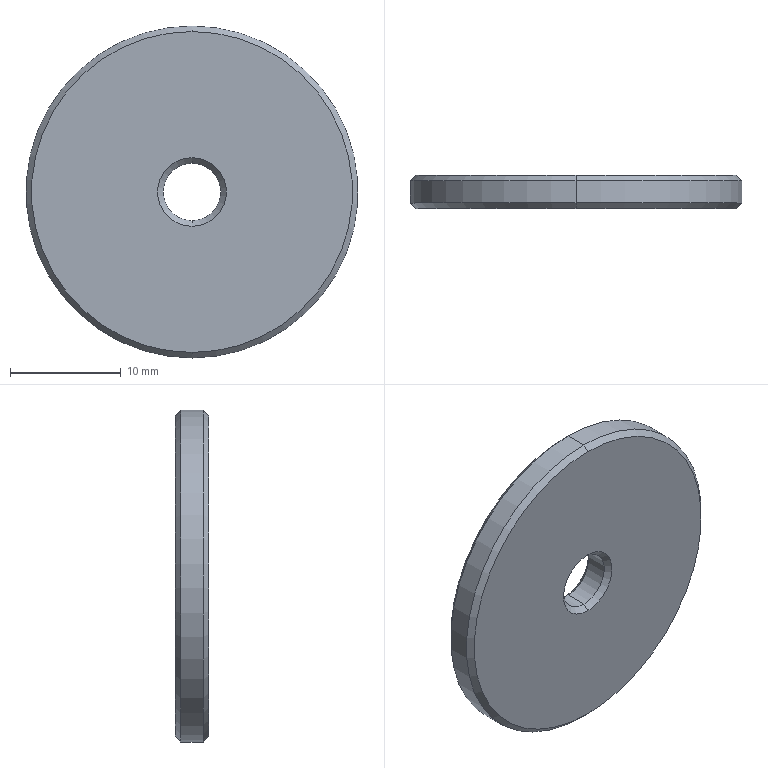Part | SolidWorks | features BaseBody 1 | 1 solid | 14 faces | box 30 x 3 x 30 mm | volume 2029 mm3 | cone 8 | cylinder 4 | plane 2 | commonest cylinder face diameters 5.2 x2 30 x2
STEP:
#1=CARTESIAN_POINT('',(0.,1.5,14.5));
#2=VERTEX_POINT('',#1);
#3=CARTESIAN_POINT('',(0.,1.5,-14.5));
#4=VERTEX_POINT('',#3);
#5=CARTESIAN_POINT('',(0.,1.5,0.));
#6=DIRECTION('',(0.,1.,0.));
#7=DIRECTION('',(0.,0.,1.));
#8=AXIS2_PLACEMENT_3D('',#5,#6,#7);
#9=CIRCLE('',#8,14.5);
#10=EDGE_CURVE('',#2,#4,#9,.T.);
#11=ORIENTED_EDGE('',*,*,#10,.F.);
#12=CARTESIAN_POINT('',(0.,1.,15.));
#13=VERTEX_POINT('',#12);
#14=CARTESIAN_POINT('',(0.,1.5,14.5));
#15=DIRECTION('',(0.,-0.7071,0.7071));
#16=VECTOR('',#15,1000.);
#17=LINE('',#14,#16);
#18=EDGE_CURVE('',#2,#13,#17,.T.);
#19=ORIENTED_EDGE('',*,*,#18,.T.);
#20=CARTESIAN_POINT('',(0.,1.,-15.));
#21=VERTEX_POINT('',#20);
#22=CARTESIAN_POINT('',(0.,1.,0.));
#23=DIRECTION('',(0.,-1.,0.));
#24=DIRECTION('',(0.,0.,1.));
#25=AXIS2_PLACEMENT_3D('',#22,#23,#24);
#26=CIRCLE('',#25,15.);
#27=EDGE_CURVE('',#21,#13,#26,.T.);
#28=ORIENTED_EDGE('',*,*,#27,.F.);
#29=CARTESIAN_POINT('',(0.,1.5,-14.5));
#30=DIRECTION('',(0.,-0.7071,-0.7071));
#31=VECTOR('',#30,1000.);
#32=LINE('',#29,#31);
#33=EDGE_CURVE('',#4,#21,#32,.T.);
#34=ORIENTED_EDGE('',*,*,#33,.F.);
#35=EDGE_LOOP('',(#11,#19,#28,#34));
#36=FACE_OUTER_BOUND('',#35,.T.);
#37=CARTESIAN_POINT('',(0.,1.5,0.));
#38=DIRECTION('',(0.,-1.,0.));
#39=DIRECTION('',(0.,0.,-1.));
#40=AXIS2_PLACEMENT_3D('',#37,#38,#39);
#41=CONICAL_SURFACE('',#40,14.5,0.7854);
#42=ADVANCED_FACE('',(#36),#41,.T.);
#43=CARTESIAN_POINT('',(0.,-1.5,-14.5));
#44=VERTEX_POINT('',#43);
#45=CARTESIAN_POINT('',(0.,-1.5,14.5));
#46=VERTEX_POINT('',#45);
#47=CARTESIAN_POINT('',(0.,-1.5,0.));
#48=DIRECTION('',(0.,-1.,0.));
#49=DIRECTION('',(0.,0.,1.));
#50=AXIS2_PLACEMENT_3D('',#47,#48,#49);
#51=CIRCLE('',#50,14.5);
#52=EDGE_CURVE('',#44,#46,#51,.T.);
#53=ORIENTED_EDGE('',*,*,#52,.F.);
#54=CARTESIAN_POINT('',(0.,-1.,-15.));
#55=VERTEX_POINT('',#54);
#56=CARTESIAN_POINT('',(0.,-1.,-15.));
#57=DIRECTION('',(0.,0.7071,-0.7071));
#58=VECTOR('',#57,1000.);
#59=LINE('',#56,#58);
#60=EDGE_CURVE('',#44,#55,#59,.T.);
#61=ORIENTED_EDGE('',*,*,#60,.T.);
#62=CARTESIAN_POINT('',(0.,-1.,15.));
#63=VERTEX_POINT('',#62);
#64=CARTESIAN_POINT('',(0.,-1.,0.));
#65=DIRECTION('',(0.,1.,0.));
#66=DIRECTION('',(0.,0.,1.));
#67=AXIS2_PLACEMENT_3D('',#64,#65,#66);
#68=CIRCLE('',#67,15.);
#69=EDGE_CURVE('',#63,#55,#68,.T.);
#70=ORIENTED_EDGE('',*,*,#69,.F.);
#71=CARTESIAN_POINT('',(0.,-1.,15.));
#72=DIRECTION('',(0.,0.7071,0.7071));
#73=VECTOR('',#72,1000.);
#74=LINE('',#71,#73);
#75=EDGE_CURVE('',#46,#63,#74,.T.);
#76=ORIENTED_EDGE('',*,*,#75,.F.);
#77=EDGE_LOOP('',(#53,#61,#70,#76));
#78=FACE_OUTER_BOUND('',#77,.T.);
#79=CARTESIAN_POINT('',(0.,-1.,0.));
#80=DIRECTION('',(0.,1.,0.));
#81=DIRECTION('',(0.,0.,1.));
#82=AXIS2_PLACEMENT_3D('',#79,#80,#81);
#83=CONICAL_SURFACE('',#82,15.,0.7854);
#84=ADVANCED_FACE('',(#78),#83,.T.);
#85=CARTESIAN_POINT('',(0.,1.,-2.6));
#86=VERTEX_POINT('',#85);
#87=CARTESIAN_POINT('',(0.,1.,2.6));
#88=VERTEX_POINT('',#87);
#89=CARTESIAN_POINT('',(0.,1.,0.));
#90=DIRECTION('',(0.,1.,0.));
#91=DIRECTION('',(0.,0.,1.));
#92=AXIS2_PLACEMENT_3D('',#89,#90,#91);
#93=CIRCLE('',#92,2.6);
#94=EDGE_CURVE('',#86,#88,#93,.T.);
#95=ORIENTED_EDGE('',*,*,#94,.F.);
#96=CARTESIAN_POINT('',(0.,1.5,-3.1));
#97=VERTEX_POINT('',#96);
#98=CARTESIAN_POINT('',(0.,1.,-2.6));
#99=DIRECTION('',(0.,0.7071,-0.7071));
#100=VECTOR('',#99,1000.);
#101=LINE('',#98,#100);
#102=EDGE_CURVE('',#86,#97,#101,.T.);
#103=ORIENTED_EDGE('',*,*,#102,.T.);
#104=CARTESIAN_POINT('',(0.,1.5,3.1));
#105=VERTEX_POINT('',#104);
#106=CARTESIAN_POINT('',(0.,1.5,0.));
#107=DIRECTION('',(0.,-1.,0.));
#108=DIRECTION('',(0.,0.,1.));
#109=AXIS2_PLACEMENT_3D('',#106,#107,#108);
#110=CIRCLE('',#109,3.1);
#111=EDGE_CURVE('',#105,#97,#110,.T.);
#112=ORIENTED_EDGE('',*,*,#111,.F.);
#113=CARTESIAN_POINT('',(0.,1.,2.6));
#114=DIRECTION('',(0.,0.7071,0.7071));
#115=VECTOR('',#114,1000.);
#116=LINE('',#113,#115);
#117=EDGE_CURVE('',#88,#105,#116,.T.);
#118=ORIENTED_EDGE('',*,*,#117,.F.);
#119=EDGE_LOOP('',(#95,#103,#112,#118));
#120=FACE_OUTER_BOUND('',#119,.T.);
#121=CARTESIAN_POINT('',(0.,1.,0.));
#122=DIRECTION('',(0.,1.,0.));
#123=DIRECTION('',(0.,0.,1.));
#124=AXIS2_PLACEMENT_3D('',#121,#122,#123);
#125=CONICAL_SURFACE('',#124,2.6,0.7854);
#126=ADVANCED_FACE('',(#120),#125,.F.);
#127=CARTESIAN_POINT('',(0.,-1.,2.6));
#128=VERTEX_POINT('',#127);
#129=CARTESIAN_POINT('',(0.,-1.,-2.6));
#130=VERTEX_POINT('',#129);
#131=CARTESIAN_POINT('',(0.,-1.,0.));
#132=DIRECTION('',(0.,-1.,0.));
#133=DIRECTION('',(0.,0.,1.));
#134=AXIS2_PLACEMENT_3D('',#131,#132,#133);
#135=CIRCLE('',#134,2.6);
#136=EDGE_CURVE('',#128,#130,#135,.T.);
#137=ORIENTED_EDGE('',*,*,#136,.F.);
#138=CARTESIAN_POINT('',(0.,-1.5,3.1));
#139=VERTEX_POINT('',#138);
#140=CARTESIAN_POINT('',(0.,-1.5,3.1));
#141=DIRECTION('',(0.,-0.7071,0.7071));
#142=VECTOR('',#141,1000.);
#143=LINE('',#140,#142);
#144=EDGE_CURVE('',#128,#139,#143,.T.);
#145=ORIENTED_EDGE('',*,*,#144,.T.);
#146=CARTESIAN_POINT('',(0.,-1.5,-3.1));
#147=VERTEX_POINT('',#146);
#148=CARTESIAN_POINT('',(0.,-1.5,0.));
#149=DIRECTION('',(0.,1.,0.));
#150=DIRECTION('',(0.,0.,1.));
#151=AXIS2_PLACEMENT_3D('',#148,#149,#150);
#152=CIRCLE('',#151,3.1);
#153=EDGE_CURVE('',#147,#139,#152,.T.);
#154=ORIENTED_EDGE('',*,*,#153,.F.);
#155=CARTESIAN_POINT('',(0.,-1.5,-3.1));
#156=DIRECTION('',(0.,-0.7071,-0.7071));
#157=VECTOR('',#156,1000.);
#158=LINE('',#155,#157);
#159=EDGE_CURVE('',#130,#147,#158,.T.);
#160=ORIENTED_EDGE('',*,*,#159,.F.);
#161=EDGE_LOOP('',(#137,#145,#154,#160));
#162=FACE_OUTER_BOUND('',#161,.T.);
#163=CARTESIAN_POINT('',(0.,-1.5,0.));
#164=DIRECTION('',(0.,-1.,0.));
#165=DIRECTION('',(0.,0.,-1.));
#166=AXIS2_PLACEMENT_3D('',#163,#164,#165);
#167=CONICAL_SURFACE('',#166,3.1,0.7854);
#168=ADVANCED_FACE('',(#162),#167,.F.);
#169=ORIENTED_EDGE('',*,*,#94,.T.);
#170=CARTESIAN_POINT('',(0.,1.5,2.6));
#171=DIRECTION('',(0.,-1.,0.));
#172=VECTOR('',#171,1000.);
#173=LINE('',#170,#172);
#174=EDGE_CURVE('',#88,#128,#173,.T.);
#175=ORIENTED_EDGE('',*,*,#174,.T.);
#176=ORIENTED_EDGE('',*,*,#136,.T.);
#177=CARTESIAN_POINT('',(0.,1.5,-2.6));
#178=DIRECTION('',(0.,-1.,0.));
#179=VECTOR('',#178,1000.);
#180=LINE('',#177,#179);
#181=EDGE_CURVE('',#86,#130,#180,.T.);
#182=ORIENTED_EDGE('',*,*,#181,.F.);
#183=EDGE_LOOP('',(#169,#175,#176,#182));
#184=FACE_OUTER_BOUND('',#183,.T.);
#185=CARTESIAN_POINT('',(0.,1.5,0.));
#186=DIRECTION('',(0.,-1.,0.));
#187=DIRECTION('',(0.,0.,-1.));
#188=AXIS2_PLACEMENT_3D('',#185,#186,#187);
#189=CYLINDRICAL_SURFACE('',#188,2.6);
#190=ADVANCED_FACE('',(#184),#189,.F.);
#191=ORIENTED_EDGE('',*,*,#27,.T.);
#192=CARTESIAN_POINT('',(0.,1.5,15.));
#193=DIRECTION('',(0.,-1.,0.));
#194=VECTOR('',#193,1000.);
#195=LINE('',#192,#194);
#196=EDGE_CURVE('',#13,#63,#195,.T.);
#197=ORIENTED_EDGE('',*,*,#196,.T.);
#198=ORIENTED_EDGE('',*,*,#69,.T.);
#199=CARTESIAN_POINT('',(0.,1.5,-15.));
#200=DIRECTION('',(0.,-1.,0.));
#201=VECTOR('',#200,1000.);
#202=LINE('',#199,#201);
#203=EDGE_CURVE('',#21,#55,#202,.T.);
#204=ORIENTED_EDGE('',*,*,#203,.F.);
#205=EDGE_LOOP('',(#191,#197,#198,#204));
#206=FACE_OUTER_BOUND('',#205,.T.);
#207=CARTESIAN_POINT('',(0.,1.5,0.));
#208=DIRECTION('',(0.,-1.,0.));
#209=DIRECTION('',(0.,0.,-1.));
#210=AXIS2_PLACEMENT_3D('',#207,#208,#209);
#211=CYLINDRICAL_SURFACE('',#210,15.);
#212=ADVANCED_FACE('',(#206),#211,.T.);
#213=ORIENTED_EDGE('',*,*,#153,.T.);
#214=CARTESIAN_POINT('',(0.,-1.5,0.));
#215=DIRECTION('',(0.,1.,0.));
#216=DIRECTION('',(0.,0.,1.));
#217=AXIS2_PLACEMENT_3D('',#214,#215,#216);
#218=CIRCLE('',#217,3.1);
#219=EDGE_CURVE('',#139,#147,#218,.T.);
#220=ORIENTED_EDGE('',*,*,#219,.T.);
#221=EDGE_LOOP('',(#213,#220));
#222=FACE_BOUND('',#221,.T.);
#223=CARTESIAN_POINT('',(0.,-1.5,0.));
#224=DIRECTION('',(0.,-1.,0.));
#225=DIRECTION('',(0.,0.,1.));
#226=AXIS2_PLACEMENT_3D('',#223,#224,#225);
#227=CIRCLE('',#226,14.5);
#228=EDGE_CURVE('',#46,#44,#227,.T.);
#229=ORIENTED_EDGE('',*,*,#228,.T.);
#230=ORIENTED_EDGE('',*,*,#52,.T.);
#231=EDGE_LOOP('',(#229,#230));
#232=FACE_OUTER_BOUND('',#231,.T.);
#233=CARTESIAN_POINT('',(0.,-1.5,0.));
#234=DIRECTION('',(0.,1.,0.));
#235=DIRECTION('',(1.,0.,0.));
#236=AXIS2_PLACEMENT_3D('',#233,#234,#235);
#237=PLANE('',#236);
#238=ADVANCED_FACE('',(#222,#232),#237,.F.);
#239=ORIENTED_EDGE('',*,*,#111,.T.);
#240=CARTESIAN_POINT('',(0.,1.5,0.));
#241=DIRECTION('',(0.,-1.,0.));
#242=DIRECTION('',(0.,0.,1.));
#243=AXIS2_PLACEMENT_3D('',#240,#241,#242);
#244=CIRCLE('',#243,3.1);
#245=EDGE_CURVE('',#97,#105,#244,.T.);
#246=ORIENTED_EDGE('',*,*,#245,.T.);
#247=EDGE_LOOP('',(#239,#246));
#248=FACE_BOUND('',#247,.T.);
#249=CARTESIAN_POINT('',(0.,1.5,0.));
#250=DIRECTION('',(0.,1.,0.));
#251=DIRECTION('',(0.,0.,1.));
#252=AXIS2_PLACEMENT_3D('',#249,#250,#251);
#253=CIRCLE('',#252,14.5);
#254=EDGE_CURVE('',#4,#2,#253,.T.);
#255=ORIENTED_EDGE('',*,*,#254,.T.);
#256=ORIENTED_EDGE('',*,*,#10,.T.);
#257=EDGE_LOOP('',(#255,#256));
#258=FACE_OUTER_BOUND('',#257,.T.);
#259=CARTESIAN_POINT('',(0.,1.5,0.));
#260=DIRECTION('',(0.,1.,0.));
#261=DIRECTION('',(1.,0.,0.));
#262=AXIS2_PLACEMENT_3D('',#259,#260,#261);
#263=PLANE('',#262);
#264=ADVANCED_FACE('',(#248,#258),#263,.T.);
#265=ORIENTED_EDGE('',*,*,#196,.F.);
#266=CARTESIAN_POINT('',(0.,1.,0.));
#267=DIRECTION('',(0.,-1.,0.));
#268=DIRECTION('',(0.,0.,1.));
#269=AXIS2_PLACEMENT_3D('',#266,#267,#268);
#270=CIRCLE('',#269,15.);
#271=EDGE_CURVE('',#13,#21,#270,.T.);
#272=ORIENTED_EDGE('',*,*,#271,.T.);
#273=ORIENTED_EDGE('',*,*,#203,.T.);
#274=CARTESIAN_POINT('',(0.,-1.,0.));
#275=DIRECTION('',(0.,1.,0.));
#276=DIRECTION('',(0.,0.,1.));
#277=AXIS2_PLACEMENT_3D('',#274,#275,#276);
#278=CIRCLE('',#277,15.);
#279=EDGE_CURVE('',#55,#63,#278,.T.);
#280=ORIENTED_EDGE('',*,*,#279,.T.);
#281=EDGE_LOOP('',(#265,#272,#273,#280));
#282=FACE_OUTER_BOUND('',#281,.T.);
#283=CARTESIAN_POINT('',(0.,1.5,0.));
#284=DIRECTION('',(0.,-1.,0.));
#285=DIRECTION('',(0.,0.,-1.));
#286=AXIS2_PLACEMENT_3D('',#283,#284,#285);
#287=CYLINDRICAL_SURFACE('',#286,15.);
#288=ADVANCED_FACE('',(#282),#287,.T.);
#289=ORIENTED_EDGE('',*,*,#174,.F.);
#290=CARTESIAN_POINT('',(0.,1.,0.));
#291=DIRECTION('',(0.,1.,0.));
#292=DIRECTION('',(0.,0.,1.));
#293=AXIS2_PLACEMENT_3D('',#290,#291,#292);
#294=CIRCLE('',#293,2.6);
#295=EDGE_CURVE('',#88,#86,#294,.T.);
#296=ORIENTED_EDGE('',*,*,#295,.T.);
#297=ORIENTED_EDGE('',*,*,#181,.T.);
#298=CARTESIAN_POINT('',(0.,-1.,0.));
#299=DIRECTION('',(0.,-1.,0.));
#300=DIRECTION('',(0.,0.,1.));
#301=AXIS2_PLACEMENT_3D('',#298,#299,#300);
#302=CIRCLE('',#301,2.6);
#303=EDGE_CURVE('',#130,#128,#302,.T.);
#304=ORIENTED_EDGE('',*,*,#303,.T.);
#305=EDGE_LOOP('',(#289,#296,#297,#304));
#306=FACE_OUTER_BOUND('',#305,.T.);
#307=CARTESIAN_POINT('',(0.,1.5,0.));
#308=DIRECTION('',(0.,-1.,0.));
#309=DIRECTION('',(0.,0.,-1.));
#310=AXIS2_PLACEMENT_3D('',#307,#308,#309);
#311=CYLINDRICAL_SURFACE('',#310,2.6);
#312=ADVANCED_FACE('',(#306),#311,.F.);
#313=ORIENTED_EDGE('',*,*,#144,.F.);
#314=ORIENTED_EDGE('',*,*,#303,.F.);
#315=ORIENTED_EDGE('',*,*,#159,.T.);
#316=ORIENTED_EDGE('',*,*,#219,.F.);
#317=EDGE_LOOP('',(#313,#314,#315,#316));
#318=FACE_OUTER_BOUND('',#317,.T.);
#319=CARTESIAN_POINT('',(0.,-1.5,0.));
#320=DIRECTION('',(0.,-1.,0.));
#321=DIRECTION('',(0.,0.,-1.));
#322=AXIS2_PLACEMENT_3D('',#319,#320,#321);
#323=CONICAL_SURFACE('',#322,3.1,0.7854);
#324=ADVANCED_FACE('',(#318),#323,.F.);
#325=ORIENTED_EDGE('',*,*,#102,.F.);
#326=ORIENTED_EDGE('',*,*,#295,.F.);
#327=ORIENTED_EDGE('',*,*,#117,.T.);
#328=ORIENTED_EDGE('',*,*,#245,.F.);
#329=EDGE_LOOP('',(#325,#326,#327,#328));
#330=FACE_OUTER_BOUND('',#329,.T.);
#331=CARTESIAN_POINT('',(0.,1.,0.));
#332=DIRECTION('',(0.,1.,0.));
#333=DIRECTION('',(0.,0.,1.));
#334=AXIS2_PLACEMENT_3D('',#331,#332,#333);
#335=CONICAL_SURFACE('',#334,2.6,0.7854);
#336=ADVANCED_FACE('',(#330),#335,.F.);
#337=ORIENTED_EDGE('',*,*,#60,.F.);
#338=ORIENTED_EDGE('',*,*,#228,.F.);
#339=ORIENTED_EDGE('',*,*,#75,.T.);
#340=ORIENTED_EDGE('',*,*,#279,.F.);
#341=EDGE_LOOP('',(#337,#338,#339,#340));
#342=FACE_OUTER_BOUND('',#341,.T.);
#343=CARTESIAN_POINT('',(0.,-1.,0.));
#344=DIRECTION('',(0.,1.,0.));
#345=DIRECTION('',(0.,0.,1.));
#346=AXIS2_PLACEMENT_3D('',#343,#344,#345);
#347=CONICAL_SURFACE('',#346,15.,0.7854);
#348=ADVANCED_FACE('',(#342),#347,.T.);
#349=ORIENTED_EDGE('',*,*,#18,.F.);
#350=ORIENTED_EDGE('',*,*,#254,.F.);
#351=ORIENTED_EDGE('',*,*,#33,.T.);
#352=ORIENTED_EDGE('',*,*,#271,.F.);
#353=EDGE_LOOP('',(#349,#350,#351,#352));
#354=FACE_OUTER_BOUND('',#353,.T.);
#355=CARTESIAN_POINT('',(0.,1.5,0.));
#356=DIRECTION('',(0.,-1.,0.));
#357=DIRECTION('',(0.,0.,-1.));
#358=AXIS2_PLACEMENT_3D('',#355,#356,#357);
#359=CONICAL_SURFACE('',#358,14.5,0.7854);
#360=ADVANCED_FACE('',(#354),#359,.T.);
#361=CLOSED_SHELL('',(#42,#84,#126,#168,#190,#212,#238,#264,#288,#312,#324,#336,#348,#360));
#362=MANIFOLD_SOLID_BREP('',#361);
#363=CARTESIAN_POINT('',(0.,0.,0.));
#364=DIRECTION('',(0.,0.,1.));
#365=DIRECTION('',(1.,0.,0.));
#366=AXIS2_PLACEMENT_3D('',#363,#364,#365);
#367=(LENGTH_UNIT()NAMED_UNIT(*)SI_UNIT(.MILLI.,.METRE.));
#368=UNCERTAINTY_MEASURE_WITH_UNIT(LENGTH_MEASURE(0.00001),#367,'','');
#369=(NAMED_UNIT(*)PLANE_ANGLE_UNIT()SI_UNIT($,.RADIAN.));
#370=(NAMED_UNIT(*)SI_UNIT($,.STERADIAN.)SOLID_ANGLE_UNIT());
#371=(GEOMETRIC_REPRESENTATION_CONTEXT(3)GLOBAL_UNCERTAINTY_ASSIGNED_CONTEXT((#368))GLOBAL_UNIT_ASSIGNED_CONTEXT((#367,#369,#370))REPRESENTATION_CONTEXT('',''));
#372=ADVANCED_BREP_SHAPE_REPRESENTATION('',(#362,#366),#371);